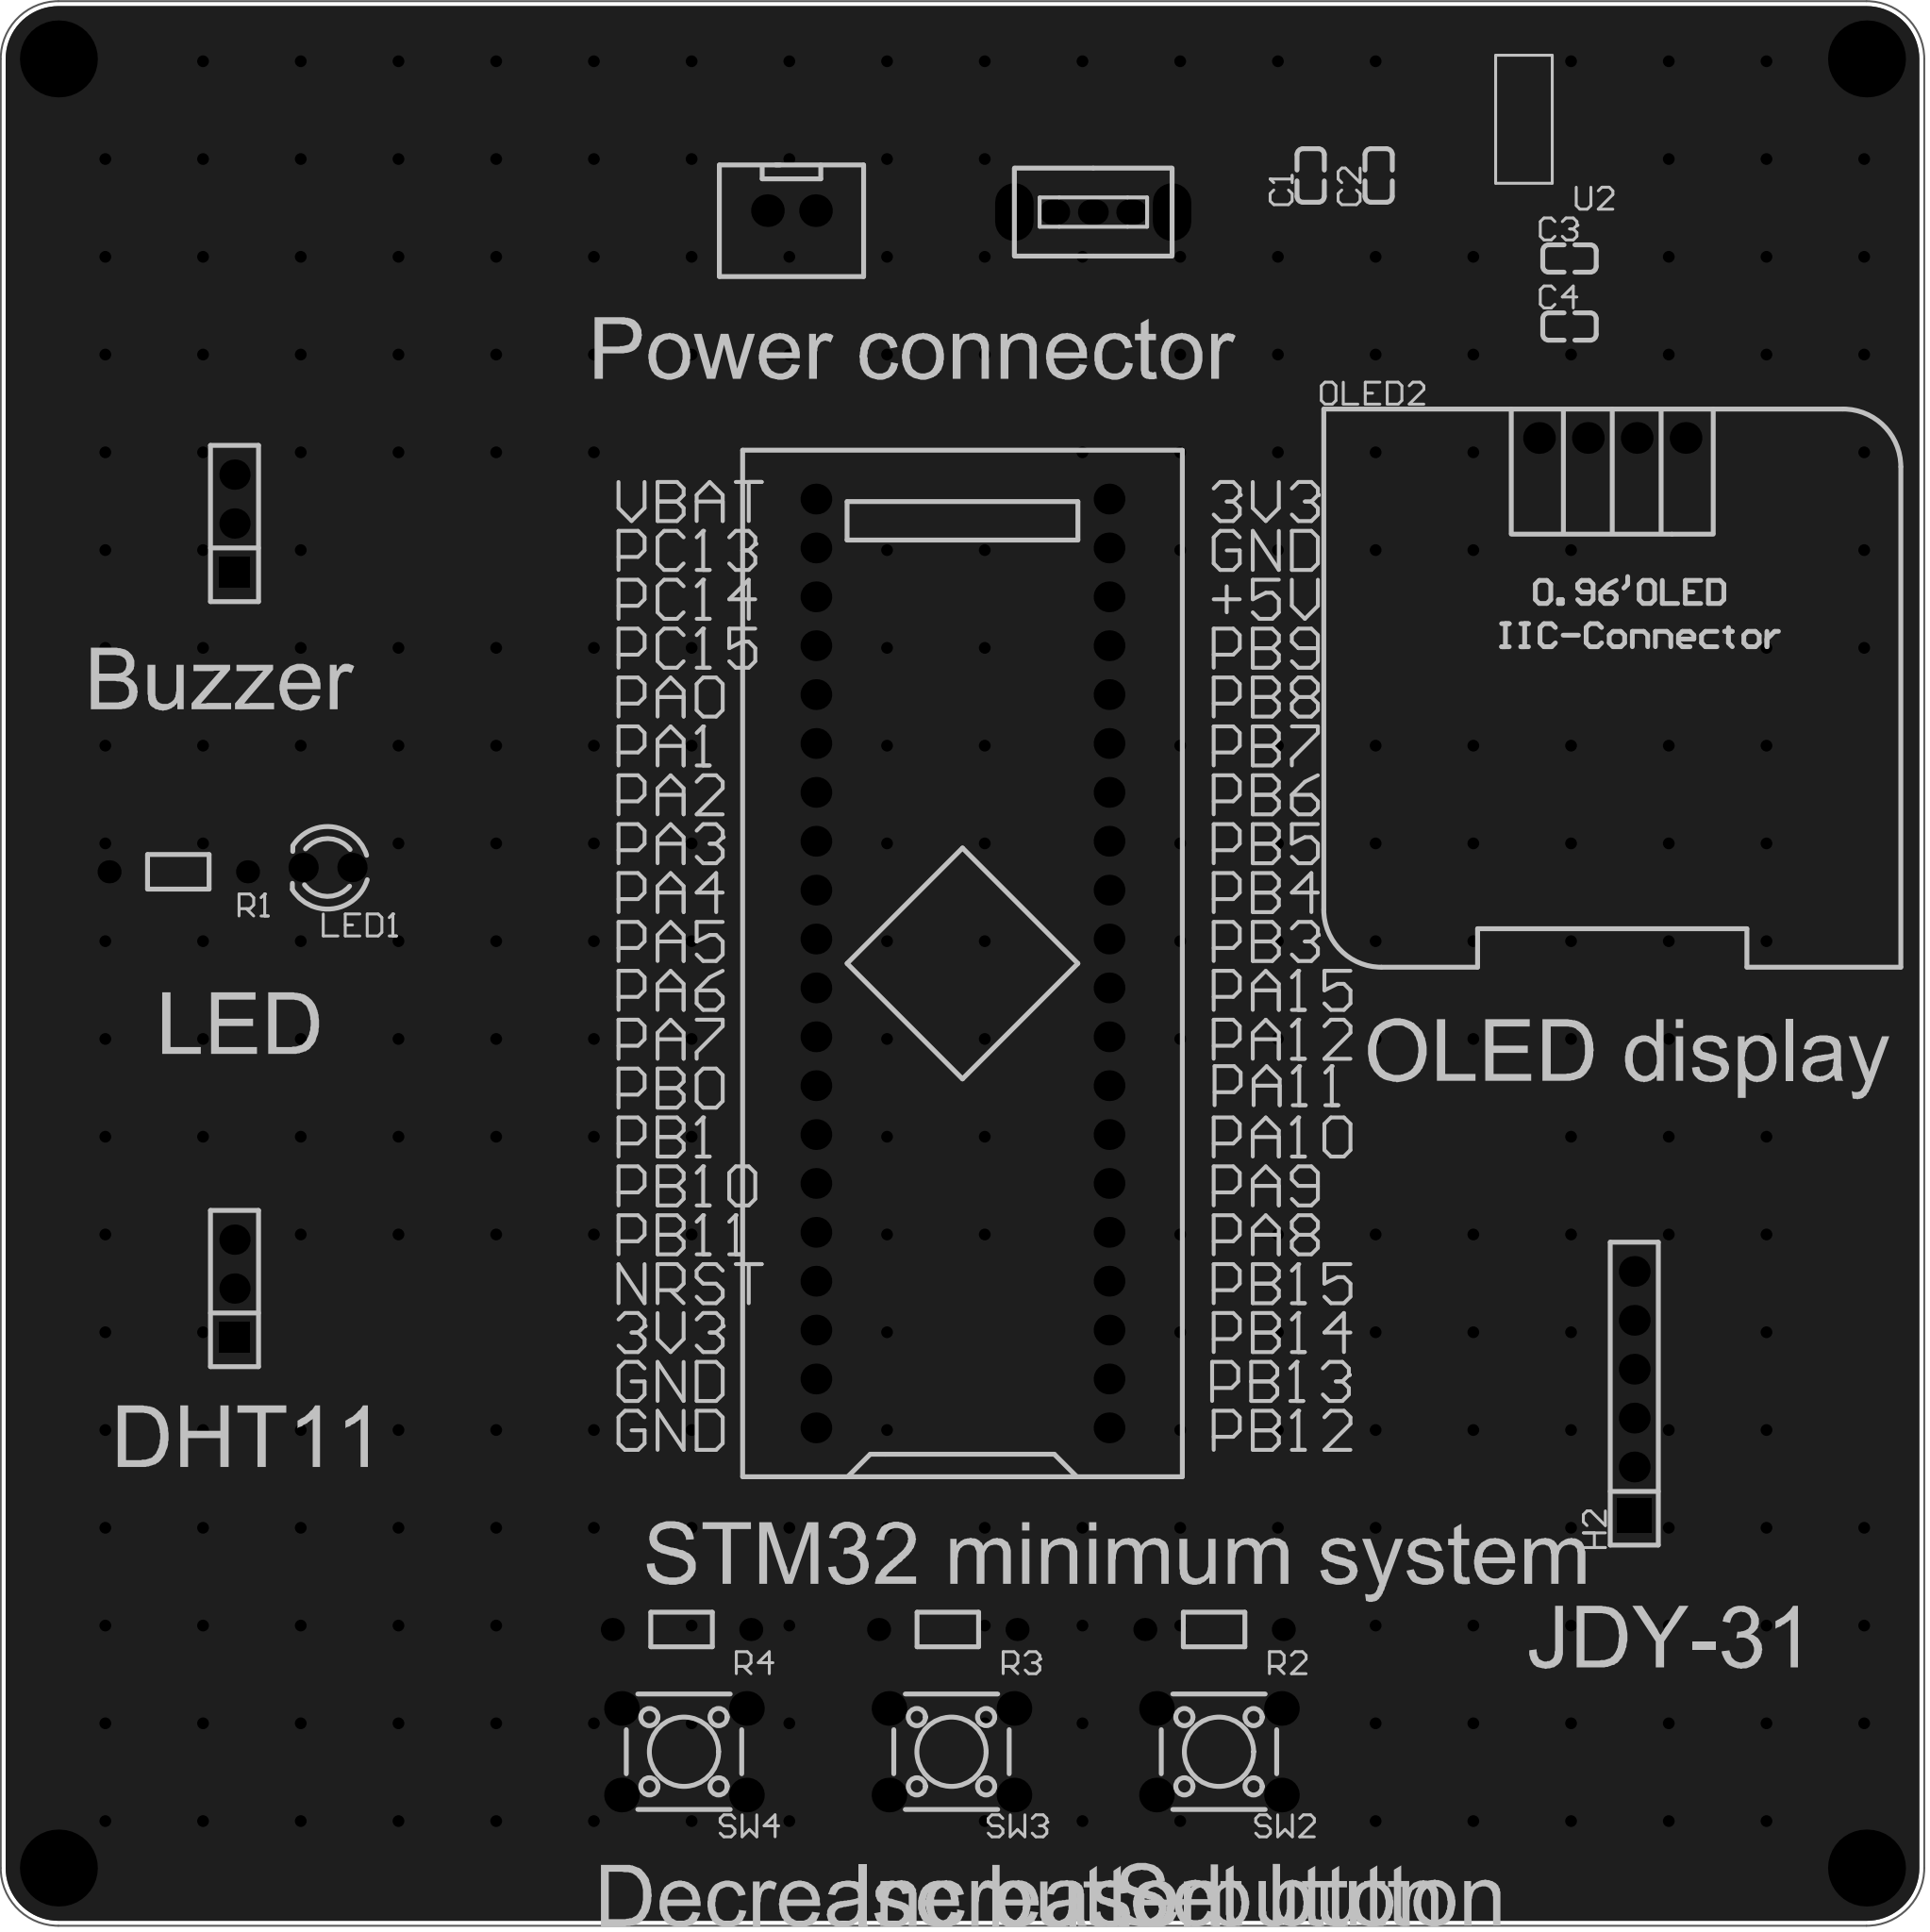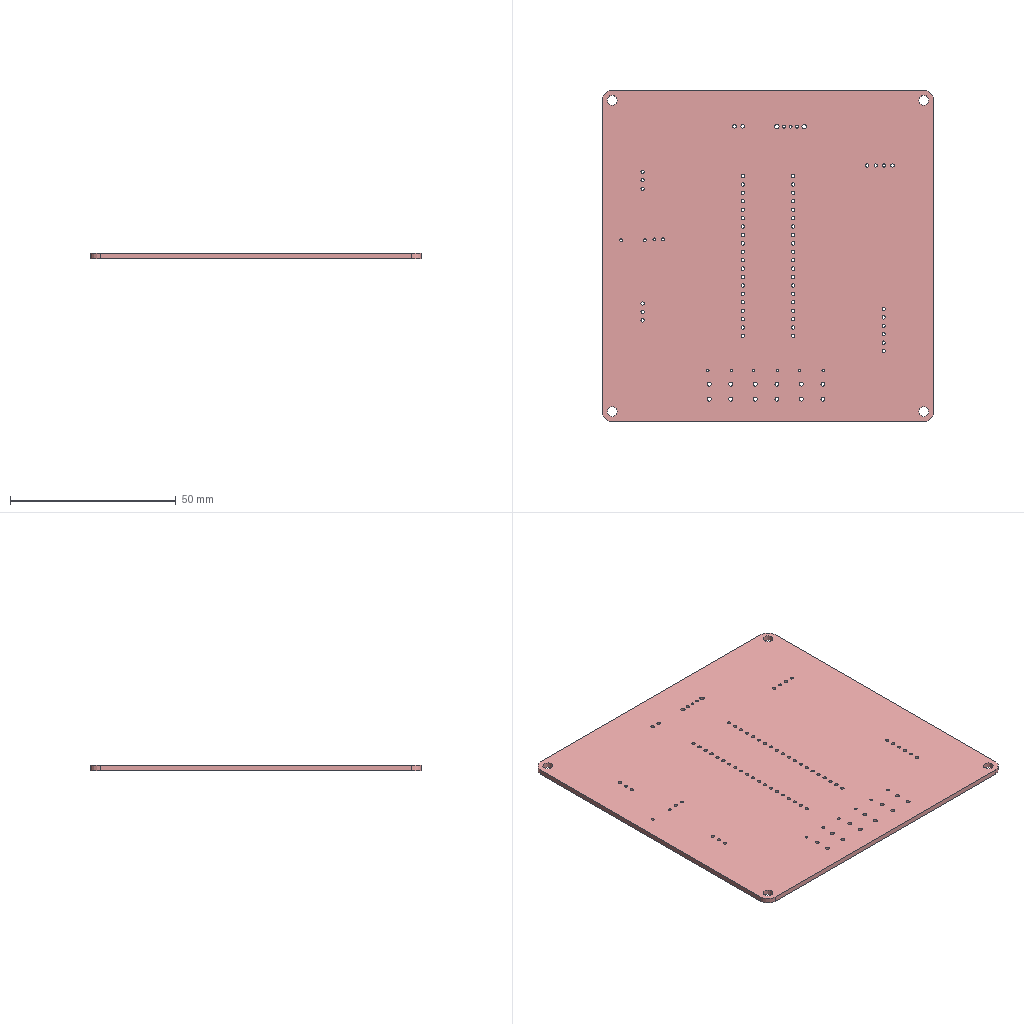Circuit board layout | Altium Designer | box 100 x 100 x 1.6 mm
Layer stack:
# Altium Designer layer stack of  (unit mm; dielectric type: 0 none, 1 core, 2 prepreg, 3 surface material)
index,name,kind,layer,copper_thickness_mm,dielectric_type,dielectric_thickness_mm,dielectric_material,dielectric_constant
0,Top Paste Mask Layer,other,,,,,,
1,Top Silkscreen Layer,other,,,,,,
2,Top Solder Mask Layer,dielectric,,,3,0.01,,3.3
3,Top Layer,copper,Top Layer,0.035,,,,
4,Dielectric1,dielectric,,,3,1.51,FR4,4.5
5,Bottom Layer,copper,Bottom Layer,0.035,,,,
6,Bottom Solder Mask Layer,dielectric,,,3,0.01,,3.3
7,Bottom Silkscreen Layer,other,,,,,,
8,Bottom Paste Mask Layer,other,,,,,,
# drill layer pairs: low layer,high layer
drill_pair,Top Layer,Bottom Layer
Part placement:
Designator,Comment,Layer,Footprint,Center-X(mm),Center-Y(mm),Rotation
U1,STM32F103C8T6-Card,TopLayer,CONN-TH_L53.3-W22.9_STM32F103C8T6-CARD,141.351,130.937,90
SW2,,TopLayer,SW-TH_4P-L6.0-W6.0-P4.50-LS6.5,154.686,89.979,180
SW3,,TopLayer,SW-TH_4P-L6.0-W6.0-P4.50-LS6.5,140.78,89.979,180
SW4,,TopLayer,SW-TH_4P-L6.0-W6.0-P4.50-LS6.5,126.873,89.979,180
CN4,XH2.54*2P_Through-hole,TopLayer,CONN-TH_2P-P2.50-XH2.54-2P,132.461,170.053,0
SW5,,TopLayer,拨动开关,148.148,169.978,180
H1,,TopLayer,HDR-TH_3P-P2.54-V-F,103.505,153.797,90
H3,,TopLayer,HDR-TH_3P-P2.54-V-F,103.505,114.046,90
H2,,TopLayer,HDR-TH_6P-P2.54-V-F,176.276,108.585,90
OLED2,,TopLayer,0.96OLED_4P,175.133,158.242,0
C1,100nF,TopLayer,C0603,159.452,171.88,90
C2,10uF,TopLayer,C0603,162.986,171.88,90
C3,100nF,TopLayer,C0603,172.907,167.566,0
C4,10uF,TopLayer,C0603,172.907,164.033,0
LED1,,TopLayer,LED_TH-3mm,108.343,135.922,180
R1,100,TopLayer,Res_1/8W,100.584,135.7,180
R2,200Ω,TopLayer,Res_1/8W,154.432,96.33,180
R3,200Ω,TopLayer,Res_1/8W,140.589,96.33,180
R4,200Ω,TopLayer,Res_1/8W,126.746,96.33,180
U2,AMS1117-3.3,TopLayer,SOT-223-3_L6.5-W3.4-P2.30-LS7.0-BR,170.44,174.802,180
Pad and via stacks:
# Altium Designer via and pad stacks of  (unit mm). Each distinct definition once, with the count of objects using it.
# via: kind,start_layer,end_layer,hole_mm,diameter_mm,mode(0 simple;1 top-mid-bottom;2 full stack),diameter_per_layer,count,example_net
# pad: kind,layer,hole_mm,hole_type(0 round;1 square;2 slot),plating,top_size,top_shape(1 round;2 rect;3 octagon;9 rounded rect),mid_size,bottom_size,mode,footprint,size_per_layer,count,example
pad,Multi-Layer,3,0,plated,4x4,1,4x4,4x4,0,,,4,1
pad,Multi-Layer,1,0,plated,1.6x1.6,1,1.6x1.6,1.6x1.6,0,CONN-TH_L53.3-W22.9_STM32F103C8T6-CARD,,40,U1.1
pad,Multi-Layer,1.2,0,plated,1.8x1.8,1,1.8x1.8,1.8x1.8,0,SW-TH_4P-L6.0-W6.0-P4.50-LS6.5,,12,SW2.1
pad,Multi-Layer,1.05,0,plated,1.7x1.7,1,1.7x1.7,1.7x1.7,0,CONN-TH_2P-P2.50-XH2.54-2P,,2,CN4.2
pad,Multi-Layer,0.8992,0,plated,1.6x1.3,1,1.6x1.3,1.6x1.3,0,\u00B2\u00A6\u00B6\u00AF\u00BF\u00AA\u00B9\u00D8,,3,SW5.1
pad,Multi-Layer,1.3,0,plated,3x1.999,1,3x1.999,3x1.999,0,\u00B2\u00A6\u00B6\u00AF\u00BF\u00AA\u00B9\u00D8,,2,SW5.4
pad,Multi-Layer,1.02,0,plated,1.575x1.575,1,1.575x1.575,1.575x1.575,0,HDR-TH_3P-P2.54-V-F,,4,H1.3
pad,Multi-Layer,1.02,0,plated,1.575x1.575,2,1.575x1.575,1.575x1.575,0,HDR-TH_3P-P2.54-V-F,,2,H1.1
pad,Multi-Layer,1.02,0,plated,1.6x1.6,1,1.6x1.6,1.6x1.6,0,HDR-TH_6P-P2.54-V-F,,5,H2.6
pad,Multi-Layer,1.02,0,plated,1.8x1.8,2,1.8x1.8,1.8x1.8,0,HDR-TH_6P-P2.54-V-F,,1,H2.1
pad,Multi-Layer,1,0,plated,1.65x1.65,1,1.65x1.65,1.65x1.65,0,0.96OLED_4P,,4,OLED2.4
pad,Multi-Layer,0.9144,0,plated,1.524x1.524,1,1.524x1.524,1.524x1.524,0,LED_TH-3mm,,2,LED1.1
pad,Multi-Layer,0.8001,0,plated,1.199x1.199,1,1.199x1.199,1.199x1.199,0,Res_1/8W,,8,R1.1
pad,Top Layer,0,0,plated,0.8x0.9,2,0.8x0.9,0.8x0.9,0,C0603,,8,C1.2
pad,Top Layer,0,0,plated,2.5x1.1,2,2.5x1.1,2.5x1.1,0,SOT-223-3_L6.5-W3.4-P2.30-LS7.0-BR,,3,U2.1
pad,Top Layer,0,0,plated,2.34x3.6,2,2.34x3.6,2.34x3.6,0,SOT-223-3_L6.5-W3.4-P2.30-LS7.0-BR,,1,U2.4
via,Top Layer,Bottom Layer,0.3048,0.61,0,,280,GND
Copper pours:
name,layer,net,type(0 solid;1 hatched;2 none)
Bottom Layer-GND,Bottom Layer,GND,0
Top Layer-GND,Top Layer,GND,0
Design rules, without the lines most boards share:
# Altium Designer design rules of  (exported by Altium Designer, unit mm)
# columns: name | kind | enabled | priority | scope1 | scope2 | descriptor | typed fields (field=value)
Copper_copperRegion_copperThickness1oz | 0 | disabled | 4 | All | All | Clearance Constraint (Gap=5.984mil) (Disabled)(All),(All) | gap=0.152
Copper_copperRegion_copperThickness1oz_1 | 63 | disabled | 4 | All | All | Board Clearance Constraint (Gap=0mil) (Disabled)(All) |
Copper_copperRegion_Copper_copperRegion | 0 | disabled | 5 | All | All | Clearance Constraint (Gap=5.984mil) (Disabled)(All),(All) | gap=0.152
Copper_copperRegion_Copper_copperRegion_1 | 63 | disabled | 5 | All | All | Board Clearance Constraint (Gap=0mil) (Disabled)(All) |
copperThickness1oz | 0 | enabled | 6 | All | All | Clearance Constraint (Gap=5.984mil) (All),(All) | gap=0.152
copperThickness1oz_1 | 63 | enabled | 6 | All | All | Board Clearance Constraint (Gap=0mil) (All) |
copperRegion_copperThickness1oz | 20 | disabled | 1 | All | All | Polygon Connect Rule(Relief Connect )(Conductor Width=10mil) (Relief Angle=90 Angle) (Entries=4) (Air Gap Width=10mil) (Disabled)(All),(All) | connect_style(0=relief,1=direct,2=none)=0 relief_conductor_width=0.254 relief_entries=4
copperRegion_Copper_copperRegion | 20 | disabled | 2 | All | All | Polygon Connect Rule(Relief Connect )(Conductor Width=10mil) (Relief Angle=90 Angle) (Entries=4) (Air Gap Width=10mil) (Disabled)(All),(All) | connect_style(0=relief,1=direct,2=none)=0 relief_conductor_width=0.254 relief_entries=4
copperRegion | 20 | enabled | 3 | All | All | Polygon Connect Rule(Relief Connect )(Conductor Width=10mil) (Relief Angle=90 Angle) (Entries=4) (Air Gap Width=10mil) (All),(All) | connect_style(0=relief,1=direct,2=none)=0 relief_conductor_width=0.254 relief_entries=4